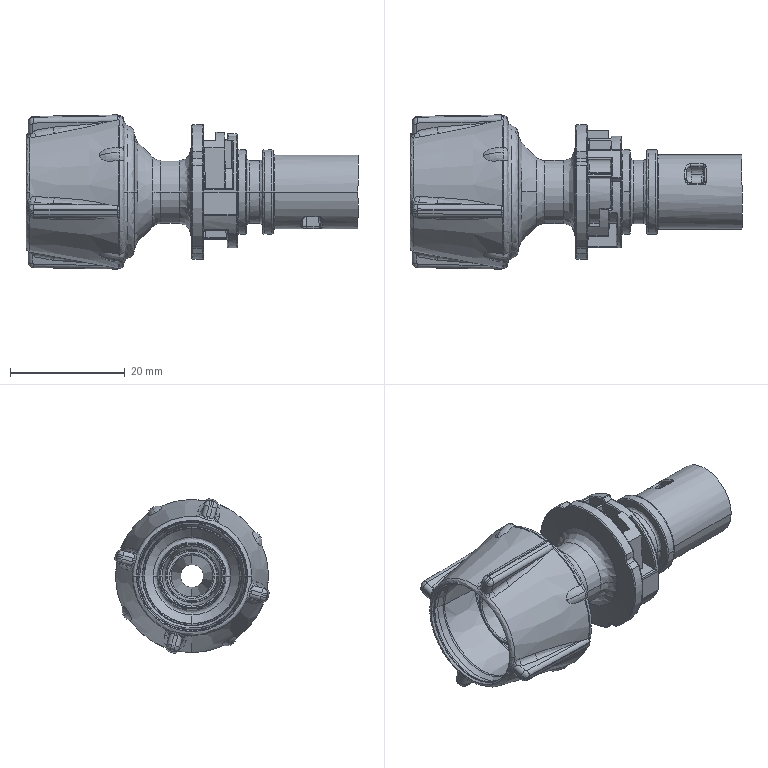Part | STEP file | Product 1 | 1 solid | 628 faces | box 57.85 x 26.867 x 26.867 mm | volume 9145 mm3 | spline 359 | cylinder 114 | plane 78 | cone 77 | commonest cylinder face diameters 0.4 x27 1.6 x18 0.3 x12 11 x11 0.5 x5 18.5 x5